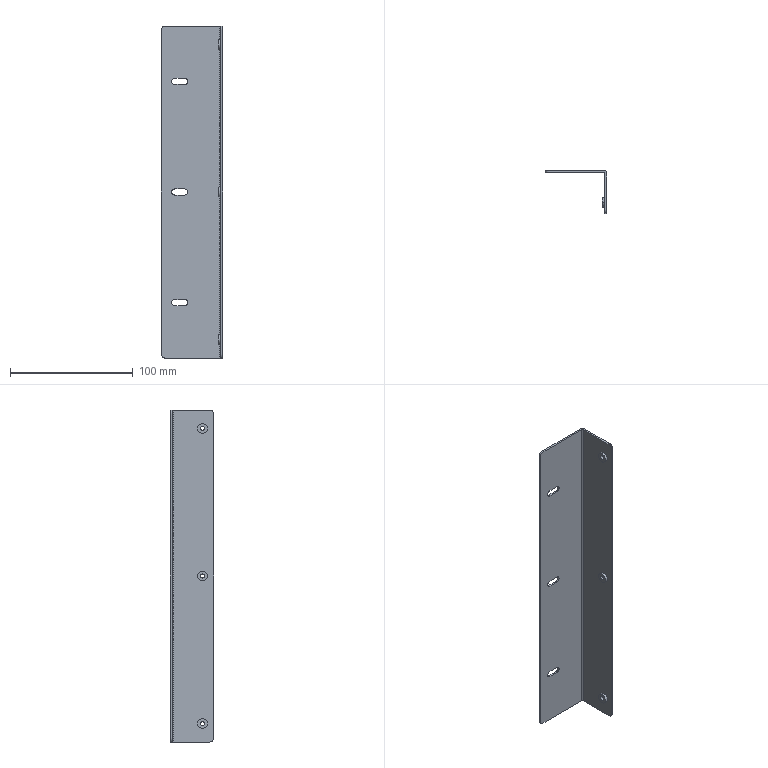Part | SolidWorks | features ICE 2, 3DProfileFeature 1, Fillet 1, FlatPattern 1, HoleWzd 1, SMBaseFlange 1, SheetMetal 1 | 1 solid | 45 faces | box 50 x 35 x 270 mm | volume 33491 mm3 | cylinder 24 | plane 21 | commonest cylinder face diameters 3.3 x6 5 x6 8 x6 6 x4 1.473 x1 4.473 x1
STEP:
#1=CARTESIAN_POINT('',(50.,-26.,-118.35));
#2=VERTEX_POINT('',#1);
#3=CARTESIAN_POINT('',(50.,-26.,-121.65));
#4=VERTEX_POINT('',#3);
#5=CARTESIAN_POINT('',(50.,-26.,-120.));
#6=DIRECTION('',(1.,0.,0.));
#7=DIRECTION('',(0.,1.,0.));
#8=AXIS2_PLACEMENT_3D('',#5,#6,#7);
#9=CIRCLE('',#8,1.65);
#10=EDGE_CURVE('',#2,#4,#9,.T.);
#11=ORIENTED_EDGE('',*,*,#10,.T.);
#12=CARTESIAN_POINT('',(46.5,-26.,-121.65));
#13=VERTEX_POINT('',#12);
#14=CARTESIAN_POINT('',(46.5,-26.,-121.65));
#15=DIRECTION('',(-1.,0.,0.));
#16=VECTOR('',#15,1000.);
#17=LINE('',#14,#16);
#18=EDGE_CURVE('',#4,#13,#17,.T.);
#19=ORIENTED_EDGE('',*,*,#18,.T.);
#20=CARTESIAN_POINT('',(46.5,-26.,-118.35));
#21=VERTEX_POINT('',#20);
#22=CARTESIAN_POINT('',(46.5,-26.,-120.));
#23=DIRECTION('',(-1.,0.,0.));
#24=DIRECTION('',(0.,0.,1.));
#25=AXIS2_PLACEMENT_3D('',#22,#23,#24);
#26=CIRCLE('',#25,1.65);
#27=EDGE_CURVE('',#13,#21,#26,.T.);
#28=ORIENTED_EDGE('',*,*,#27,.T.);
#29=CARTESIAN_POINT('',(46.5,-26.,-118.35));
#30=DIRECTION('',(-1.,0.,0.));
#31=VECTOR('',#30,1000.);
#32=LINE('',#29,#31);
#33=EDGE_CURVE('',#2,#21,#32,.T.);
#34=ORIENTED_EDGE('',*,*,#33,.F.);
#35=EDGE_LOOP('',(#11,#19,#28,#34));
#36=FACE_OUTER_BOUND('',#35,.T.);
#37=CARTESIAN_POINT('',(46.5,-26.,-120.));
#38=DIRECTION('',(-1.,0.,0.));
#39=DIRECTION('',(0.,0.,1.));
#40=AXIS2_PLACEMENT_3D('',#37,#38,#39);
#41=CYLINDRICAL_SURFACE('',#40,1.65);
#42=ADVANCED_FACE('',(#36),#41,.F.);
#43=CARTESIAN_POINT('',(50.,-26.,1.65));
#44=VERTEX_POINT('',#43);
#45=CARTESIAN_POINT('',(50.,-26.,-1.65));
#46=VERTEX_POINT('',#45);
#47=CARTESIAN_POINT('',(50.,-26.,0.));
#48=DIRECTION('',(1.,0.,0.));
#49=DIRECTION('',(0.,1.,0.));
#50=AXIS2_PLACEMENT_3D('',#47,#48,#49);
#51=CIRCLE('',#50,1.65);
#52=EDGE_CURVE('',#44,#46,#51,.T.);
#53=ORIENTED_EDGE('',*,*,#52,.T.);
#54=CARTESIAN_POINT('',(46.5,-26.,-1.65));
#55=VERTEX_POINT('',#54);
#56=CARTESIAN_POINT('',(46.5,-26.,-1.65));
#57=DIRECTION('',(-1.,0.,0.));
#58=VECTOR('',#57,1000.);
#59=LINE('',#56,#58);
#60=EDGE_CURVE('',#46,#55,#59,.T.);
#61=ORIENTED_EDGE('',*,*,#60,.T.);
#62=CARTESIAN_POINT('',(46.5,-26.,1.65));
#63=VERTEX_POINT('',#62);
#64=CARTESIAN_POINT('',(46.5,-26.,0.));
#65=DIRECTION('',(-1.,0.,0.));
#66=DIRECTION('',(0.,0.,1.));
#67=AXIS2_PLACEMENT_3D('',#64,#65,#66);
#68=CIRCLE('',#67,1.65);
#69=EDGE_CURVE('',#55,#63,#68,.T.);
#70=ORIENTED_EDGE('',*,*,#69,.T.);
#71=CARTESIAN_POINT('',(46.5,-26.,1.65));
#72=DIRECTION('',(-1.,0.,0.));
#73=VECTOR('',#72,1000.);
#74=LINE('',#71,#73);
#75=EDGE_CURVE('',#44,#63,#74,.T.);
#76=ORIENTED_EDGE('',*,*,#75,.F.);
#77=EDGE_LOOP('',(#53,#61,#70,#76));
#78=FACE_OUTER_BOUND('',#77,.T.);
#79=CARTESIAN_POINT('',(46.5,-26.,0.));
#80=DIRECTION('',(-1.,0.,0.));
#81=DIRECTION('',(0.,0.,1.));
#82=AXIS2_PLACEMENT_3D('',#79,#80,#81);
#83=CYLINDRICAL_SURFACE('',#82,1.65);
#84=ADVANCED_FACE('',(#78),#83,.F.);
#85=CARTESIAN_POINT('',(50.,-26.,121.65));
#86=VERTEX_POINT('',#85);
#87=CARTESIAN_POINT('',(50.,-26.,118.35));
#88=VERTEX_POINT('',#87);
#89=CARTESIAN_POINT('',(50.,-26.,120.));
#90=DIRECTION('',(1.,0.,0.));
#91=DIRECTION('',(0.,1.,0.));
#92=AXIS2_PLACEMENT_3D('',#89,#90,#91);
#93=CIRCLE('',#92,1.65);
#94=EDGE_CURVE('',#86,#88,#93,.T.);
#95=ORIENTED_EDGE('',*,*,#94,.T.);
#96=CARTESIAN_POINT('',(46.5,-26.,118.35));
#97=VERTEX_POINT('',#96);
#98=CARTESIAN_POINT('',(46.5,-26.,118.35));
#99=DIRECTION('',(-1.,0.,0.));
#100=VECTOR('',#99,1000.);
#101=LINE('',#98,#100);
#102=EDGE_CURVE('',#88,#97,#101,.T.);
#103=ORIENTED_EDGE('',*,*,#102,.T.);
#104=CARTESIAN_POINT('',(46.5,-26.,121.65));
#105=VERTEX_POINT('',#104);
#106=CARTESIAN_POINT('',(46.5,-26.,120.));
#107=DIRECTION('',(-1.,0.,0.));
#108=DIRECTION('',(0.,0.,1.));
#109=AXIS2_PLACEMENT_3D('',#106,#107,#108);
#110=CIRCLE('',#109,1.65);
#111=EDGE_CURVE('',#97,#105,#110,.T.);
#112=ORIENTED_EDGE('',*,*,#111,.T.);
#113=CARTESIAN_POINT('',(46.5,-26.,121.65));
#114=DIRECTION('',(-1.,0.,0.));
#115=VECTOR('',#114,1000.);
#116=LINE('',#113,#115);
#117=EDGE_CURVE('',#86,#105,#116,.T.);
#118=ORIENTED_EDGE('',*,*,#117,.F.);
#119=EDGE_LOOP('',(#95,#103,#112,#118));
#120=FACE_OUTER_BOUND('',#119,.T.);
#121=CARTESIAN_POINT('',(46.5,-26.,120.));
#122=DIRECTION('',(-1.,0.,0.));
#123=DIRECTION('',(0.,0.,1.));
#124=AXIS2_PLACEMENT_3D('',#121,#122,#123);
#125=CYLINDRICAL_SURFACE('',#124,1.65);
#126=ADVANCED_FACE('',(#120),#125,.F.);
#127=CARTESIAN_POINT('',(46.5,-26.,-124.));
#128=VERTEX_POINT('',#127);
#129=CARTESIAN_POINT('',(46.5,-26.,-116.));
#130=VERTEX_POINT('',#129);
#131=CARTESIAN_POINT('',(46.5,-26.,-120.));
#132=DIRECTION('',(1.,0.,0.));
#133=DIRECTION('',(0.,0.,1.));
#134=AXIS2_PLACEMENT_3D('',#131,#132,#133);
#135=CIRCLE('',#134,4.);
#136=EDGE_CURVE('',#128,#130,#135,.T.);
#137=ORIENTED_EDGE('',*,*,#136,.T.);
#138=CARTESIAN_POINT('',(48.5,-26.,-116.));
#139=VERTEX_POINT('',#138);
#140=CARTESIAN_POINT('',(46.5,-26.,-116.));
#141=DIRECTION('',(1.,0.,0.));
#142=VECTOR('',#141,1000.);
#143=LINE('',#140,#142);
#144=EDGE_CURVE('',#130,#139,#143,.T.);
#145=ORIENTED_EDGE('',*,*,#144,.T.);
#146=CARTESIAN_POINT('',(48.5,-26.,-124.));
#147=VERTEX_POINT('',#146);
#148=CARTESIAN_POINT('',(48.5,-26.,-120.));
#149=DIRECTION('',(1.,0.,0.));
#150=DIRECTION('',(0.,1.,0.));
#151=AXIS2_PLACEMENT_3D('',#148,#149,#150);
#152=CIRCLE('',#151,4.);
#153=EDGE_CURVE('',#147,#139,#152,.T.);
#154=ORIENTED_EDGE('',*,*,#153,.F.);
#155=CARTESIAN_POINT('',(46.5,-26.,-124.));
#156=DIRECTION('',(1.,0.,0.));
#157=VECTOR('',#156,1000.);
#158=LINE('',#155,#157);
#159=EDGE_CURVE('',#128,#147,#158,.T.);
#160=ORIENTED_EDGE('',*,*,#159,.F.);
#161=EDGE_LOOP('',(#137,#145,#154,#160));
#162=FACE_OUTER_BOUND('',#161,.T.);
#163=CARTESIAN_POINT('',(46.5,-26.,-120.));
#164=DIRECTION('',(1.,0.,0.));
#165=DIRECTION('',(0.,0.,-1.));
#166=AXIS2_PLACEMENT_3D('',#163,#164,#165);
#167=CYLINDRICAL_SURFACE('',#166,4.);
#168=ADVANCED_FACE('',(#162),#167,.T.);
#169=CARTESIAN_POINT('',(46.5,-26.,116.));
#170=VERTEX_POINT('',#169);
#171=CARTESIAN_POINT('',(46.5,-26.,124.));
#172=VERTEX_POINT('',#171);
#173=CARTESIAN_POINT('',(46.5,-26.,120.));
#174=DIRECTION('',(1.,0.,0.));
#175=DIRECTION('',(0.,0.,-1.));
#176=AXIS2_PLACEMENT_3D('',#173,#174,#175);
#177=CIRCLE('',#176,4.);
#178=EDGE_CURVE('',#170,#172,#177,.T.);
#179=ORIENTED_EDGE('',*,*,#178,.T.);
#180=CARTESIAN_POINT('',(48.5,-26.,124.));
#181=VERTEX_POINT('',#180);
#182=CARTESIAN_POINT('',(46.5,-26.,124.));
#183=DIRECTION('',(1.,0.,0.));
#184=VECTOR('',#183,1000.);
#185=LINE('',#182,#184);
#186=EDGE_CURVE('',#172,#181,#185,.T.);
#187=ORIENTED_EDGE('',*,*,#186,.T.);
#188=CARTESIAN_POINT('',(48.5,-26.,116.));
#189=VERTEX_POINT('',#188);
#190=CARTESIAN_POINT('',(48.5,-26.,120.));
#191=DIRECTION('',(1.,0.,0.));
#192=DIRECTION('',(0.,1.,0.));
#193=AXIS2_PLACEMENT_3D('',#190,#191,#192);
#194=CIRCLE('',#193,4.);
#195=EDGE_CURVE('',#189,#181,#194,.T.);
#196=ORIENTED_EDGE('',*,*,#195,.F.);
#197=CARTESIAN_POINT('',(46.5,-26.,116.));
#198=DIRECTION('',(1.,0.,0.));
#199=VECTOR('',#198,1000.);
#200=LINE('',#197,#199);
#201=EDGE_CURVE('',#170,#189,#200,.T.);
#202=ORIENTED_EDGE('',*,*,#201,.F.);
#203=EDGE_LOOP('',(#179,#187,#196,#202));
#204=FACE_OUTER_BOUND('',#203,.T.);
#205=CARTESIAN_POINT('',(46.5,-26.,120.));
#206=DIRECTION('',(1.,0.,0.));
#207=DIRECTION('',(0.,0.,-1.));
#208=AXIS2_PLACEMENT_3D('',#205,#206,#207);
#209=CYLINDRICAL_SURFACE('',#208,4.);
#210=ADVANCED_FACE('',(#204),#209,.T.);
#211=CARTESIAN_POINT('',(46.5,-26.,-4.));
#212=VERTEX_POINT('',#211);
#213=CARTESIAN_POINT('',(46.5,-26.,4.));
#214=VERTEX_POINT('',#213);
#215=CARTESIAN_POINT('',(46.5,-26.,0.));
#216=DIRECTION('',(1.,0.,0.));
#217=DIRECTION('',(0.,0.,-1.));
#218=AXIS2_PLACEMENT_3D('',#215,#216,#217);
#219=CIRCLE('',#218,4.);
#220=EDGE_CURVE('',#212,#214,#219,.T.);
#221=ORIENTED_EDGE('',*,*,#220,.T.);
#222=CARTESIAN_POINT('',(48.5,-26.,4.));
#223=VERTEX_POINT('',#222);
#224=CARTESIAN_POINT('',(46.5,-26.,4.));
#225=DIRECTION('',(1.,0.,0.));
#226=VECTOR('',#225,1000.);
#227=LINE('',#224,#226);
#228=EDGE_CURVE('',#214,#223,#227,.T.);
#229=ORIENTED_EDGE('',*,*,#228,.T.);
#230=CARTESIAN_POINT('',(48.5,-26.,-4.));
#231=VERTEX_POINT('',#230);
#232=CARTESIAN_POINT('',(48.5,-26.,0.));
#233=DIRECTION('',(1.,0.,0.));
#234=DIRECTION('',(0.,1.,0.));
#235=AXIS2_PLACEMENT_3D('',#232,#233,#234);
#236=CIRCLE('',#235,4.);
#237=EDGE_CURVE('',#231,#223,#236,.T.);
#238=ORIENTED_EDGE('',*,*,#237,.F.);
#239=CARTESIAN_POINT('',(46.5,-26.,-4.));
#240=DIRECTION('',(1.,0.,0.));
#241=VECTOR('',#240,1000.);
#242=LINE('',#239,#241);
#243=EDGE_CURVE('',#212,#231,#242,.T.);
#244=ORIENTED_EDGE('',*,*,#243,.F.);
#245=EDGE_LOOP('',(#221,#229,#238,#244));
#246=FACE_OUTER_BOUND('',#245,.T.);
#247=CARTESIAN_POINT('',(46.5,-26.,0.));
#248=DIRECTION('',(1.,0.,0.));
#249=DIRECTION('',(0.,0.,-1.));
#250=AXIS2_PLACEMENT_3D('',#247,#248,#249);
#251=CYLINDRICAL_SURFACE('',#250,4.);
#252=ADVANCED_FACE('',(#246),#251,.T.);
#253=ORIENTED_EDGE('',*,*,#178,.F.);
#254=CARTESIAN_POINT('',(46.5,-26.,120.));
#255=DIRECTION('',(1.,0.,0.));
#256=DIRECTION('',(0.,0.,-1.));
#257=AXIS2_PLACEMENT_3D('',#254,#255,#256);
#258=CIRCLE('',#257,4.);
#259=EDGE_CURVE('',#172,#170,#258,.T.);
#260=ORIENTED_EDGE('',*,*,#259,.F.);
#261=EDGE_LOOP('',(#253,#260));
#262=FACE_OUTER_BOUND('',#261,.T.);
#263=CARTESIAN_POINT('',(46.5,-26.,120.));
#264=DIRECTION('',(-1.,0.,0.));
#265=DIRECTION('',(0.,0.,1.));
#266=AXIS2_PLACEMENT_3D('',#263,#264,#265);
#267=CIRCLE('',#266,1.65);
#268=EDGE_CURVE('',#105,#97,#267,.T.);
#269=ORIENTED_EDGE('',*,*,#268,.F.);
#270=ORIENTED_EDGE('',*,*,#111,.F.);
#271=EDGE_LOOP('',(#269,#270));
#272=FACE_BOUND('',#271,.T.);
#273=CARTESIAN_POINT('',(46.5,-26.,120.));
#274=DIRECTION('',(1.,0.,0.));
#275=DIRECTION('',(0.,0.,-1.));
#276=AXIS2_PLACEMENT_3D('',#273,#274,#275);
#277=PLANE('',#276);
#278=ADVANCED_FACE('',(#262,#272),#277,.F.);
#279=CARTESIAN_POINT('',(0.,0.,132.));
#280=VERTEX_POINT('',#279);
#281=CARTESIAN_POINT('',(0.,0.,-132.));
#282=VERTEX_POINT('',#281);
#283=CARTESIAN_POINT('',(0.,0.,135.));
#284=DIRECTION('',(0.,0.,-1.));
#285=VECTOR('',#284,1000.);
#286=LINE('',#283,#285);
#287=EDGE_CURVE('',#280,#282,#286,.T.);
#288=ORIENTED_EDGE('',*,*,#287,.F.);
#289=CARTESIAN_POINT('',(3.,0.,135.));
#290=VERTEX_POINT('',#289);
#291=CARTESIAN_POINT('',(3.,0.,132.));
#292=DIRECTION('',(0.,1.,0.));
#293=DIRECTION('',(0.,0.,1.));
#294=AXIS2_PLACEMENT_3D('',#291,#292,#293);
#295=CIRCLE('',#294,3.);
#296=EDGE_CURVE('',#280,#290,#295,.T.);
#297=ORIENTED_EDGE('',*,*,#296,.T.);
#298=CARTESIAN_POINT('',(47.763,0.,135.));
#299=VERTEX_POINT('',#298);
#300=CARTESIAN_POINT('',(0.,0.,135.));
#301=DIRECTION('',(1.,0.,0.));
#302=VECTOR('',#301,1000.);
#303=LINE('',#300,#302);
#304=EDGE_CURVE('',#290,#299,#303,.T.);
#305=ORIENTED_EDGE('',*,*,#304,.T.);
#306=CARTESIAN_POINT('',(47.763,0.,-135.));
#307=VERTEX_POINT('',#306);
#308=CARTESIAN_POINT('',(47.763,0.,135.));
#309=DIRECTION('',(0.,0.,-1.));
#310=VECTOR('',#309,1000.);
#311=LINE('',#308,#310);
#312=EDGE_CURVE('',#299,#307,#311,.T.);
#313=ORIENTED_EDGE('',*,*,#312,.T.);
#314=CARTESIAN_POINT('',(3.,0.,-135.));
#315=VERTEX_POINT('',#314);
#316=CARTESIAN_POINT('',(0.,0.,-135.));
#317=DIRECTION('',(1.,0.,0.));
#318=VECTOR('',#317,1000.);
#319=LINE('',#316,#318);
#320=EDGE_CURVE('',#315,#307,#319,.T.);
#321=ORIENTED_EDGE('',*,*,#320,.F.);
#322=CARTESIAN_POINT('',(3.,0.,-132.));
#323=DIRECTION('',(0.,1.,0.));
#324=DIRECTION('',(0.,0.,1.));
#325=AXIS2_PLACEMENT_3D('',#322,#323,#324);
#326=CIRCLE('',#325,3.);
#327=EDGE_CURVE('',#315,#282,#326,.T.);
#328=ORIENTED_EDGE('',*,*,#327,.T.);
#329=EDGE_LOOP('',(#288,#297,#305,#313,#321,#328));
#330=FACE_OUTER_BOUND('',#329,.T.);
#331=CARTESIAN_POINT('',(11.,0.,87.5));
#332=VERTEX_POINT('',#331);
#333=CARTESIAN_POINT('',(19.,0.,87.5));
#334=VERTEX_POINT('',#333);
#335=CARTESIAN_POINT('',(19.,0.,87.5));
#336=DIRECTION('',(1.,0.,0.));
#337=VECTOR('',#336,1000.);
#338=LINE('',#335,#337);
#339=EDGE_CURVE('',#332,#334,#338,.T.);
#340=ORIENTED_EDGE('',*,*,#339,.T.);
#341=CARTESIAN_POINT('',(19.,0.,92.5));
#342=VERTEX_POINT('',#341);
#343=CARTESIAN_POINT('',(19.,0.,90.));
#344=DIRECTION('',(0.,-1.,0.));
#345=DIRECTION('',(0.,0.,1.));
#346=AXIS2_PLACEMENT_3D('',#343,#344,#345);
#347=CIRCLE('',#346,2.5);
#348=EDGE_CURVE('',#334,#342,#347,.T.);
#349=ORIENTED_EDGE('',*,*,#348,.T.);
#350=CARTESIAN_POINT('',(11.,0.,92.5));
#351=VERTEX_POINT('',#350);
#352=CARTESIAN_POINT('',(19.,0.,92.5));
#353=DIRECTION('',(-1.,0.,0.));
#354=VECTOR('',#353,1000.);
#355=LINE('',#352,#354);
#356=EDGE_CURVE('',#342,#351,#355,.T.);
#357=ORIENTED_EDGE('',*,*,#356,.T.);
#358=CARTESIAN_POINT('',(11.,0.,90.));
#359=DIRECTION('',(0.,-1.,0.));
#360=DIRECTION('',(0.,0.,1.));
#361=AXIS2_PLACEMENT_3D('',#358,#359,#360);
#362=CIRCLE('',#361,2.5);
#363=EDGE_CURVE('',#351,#332,#362,.T.);
#364=ORIENTED_EDGE('',*,*,#363,.T.);
#365=EDGE_LOOP('',(#340,#349,#357,#364));
#366=FACE_BOUND('',#365,.T.);
#367=CARTESIAN_POINT('',(11.,0.,-2.5));
#368=VERTEX_POINT('',#367);
#369=CARTESIAN_POINT('',(19.,0.,-2.5));
#370=VERTEX_POINT('',#369);
#371=CARTESIAN_POINT('',(19.,0.,-2.5));
#372=DIRECTION('',(1.,0.,0.));
#373=VECTOR('',#372,1000.);
#374=LINE('',#371,#373);
#375=EDGE_CURVE('',#368,#370,#374,.T.);
#376=ORIENTED_EDGE('',*,*,#375,.T.);
#377=CARTESIAN_POINT('',(19.,0.,2.5));
#378=VERTEX_POINT('',#377);
#379=CARTESIAN_POINT('',(19.,0.,0.));
#380=DIRECTION('',(0.,-1.,0.));
#381=DIRECTION('',(0.,0.,-1.));
#382=AXIS2_PLACEMENT_3D('',#379,#380,#381);
#383=CIRCLE('',#382,2.5);
#384=EDGE_CURVE('',#370,#378,#383,.T.);
#385=ORIENTED_EDGE('',*,*,#384,.T.);
#386=CARTESIAN_POINT('',(11.,0.,2.5));
#387=VERTEX_POINT('',#386);
#388=CARTESIAN_POINT('',(19.,0.,2.5));
#389=DIRECTION('',(-1.,0.,0.));
#390=VECTOR('',#389,1000.);
#391=LINE('',#388,#390);
#392=EDGE_CURVE('',#378,#387,#391,.T.);
#393=ORIENTED_EDGE('',*,*,#392,.T.);
#394=CARTESIAN_POINT('',(11.,0.,0.));
#395=DIRECTION('',(0.,-1.,0.));
#396=DIRECTION('',(0.,0.,-1.));
#397=AXIS2_PLACEMENT_3D('',#394,#395,#396);
#398=CIRCLE('',#397,2.5);
#399=EDGE_CURVE('',#387,#368,#398,.T.);
#400=ORIENTED_EDGE('',*,*,#399,.T.);
#401=EDGE_LOOP('',(#376,#385,#393,#400));
#402=FACE_BOUND('',#401,.T.);
#403=CARTESIAN_POINT('',(11.,0.,-92.5));
#404=VERTEX_POINT('',#403);
#405=CARTESIAN_POINT('',(19.,0.,-92.5));
#406=VERTEX_POINT('',#405);
#407=CARTESIAN_POINT('',(19.,0.,-92.5));
#408=DIRECTION('',(1.,0.,0.));
#409=VECTOR('',#408,1000.);
#410=LINE('',#407,#409);
#411=EDGE_CURVE('',#404,#406,#410,.T.);
#412=ORIENTED_EDGE('',*,*,#411,.T.);
#413=CARTESIAN_POINT('',(19.,0.,-87.5));
#414=VERTEX_POINT('',#413);
#415=CARTESIAN_POINT('',(19.,0.,-90.));
#416=DIRECTION('',(0.,-1.,0.));
#417=DIRECTION('',(0.,0.,-1.));
#418=AXIS2_PLACEMENT_3D('',#415,#416,#417);
#419=CIRCLE('',#418,2.5);
#420=EDGE_CURVE('',#406,#414,#419,.T.);
#421=ORIENTED_EDGE('',*,*,#420,.T.);
#422=CARTESIAN_POINT('',(11.,0.,-87.5));
#423=VERTEX_POINT('',#422);
#424=CARTESIAN_POINT('',(19.,0.,-87.5));
#425=DIRECTION('',(-1.,0.,0.));
#426=VECTOR('',#425,1000.);
#427=LINE('',#424,#426);
#428=EDGE_CURVE('',#414,#423,#427,.T.);
#429=ORIENTED_EDGE('',*,*,#428,.T.);
#430=CARTESIAN_POINT('',(11.,0.,-90.));
#431=DIRECTION('',(0.,-1.,0.));
#432=DIRECTION('',(0.,0.,-1.));
#433=AXIS2_PLACEMENT_3D('',#430,#431,#432);
#434=CIRCLE('',#433,2.5);
#435=EDGE_CURVE('',#423,#404,#434,.T.);
#436=ORIENTED_EDGE('',*,*,#435,.T.);
#437=EDGE_LOOP('',(#412,#421,#429,#436));
#438=FACE_BOUND('',#437,.T.);
#439=CARTESIAN_POINT('',(0.,0.,135.));
#440=DIRECTION('',(0.,1.,0.));
#441=DIRECTION('',(0.,0.,1.));
#442=AXIS2_PLACEMENT_3D('',#439,#440,#441);
#443=PLANE('',#442);
#444=ADVANCED_FACE('',(#330,#366,#402,#438),#443,.T.);
#445=CARTESIAN_POINT('',(19.,-1.5,-2.5));
#446=VERTEX_POINT('',#445);
#447=CARTESIAN_POINT('',(19.,-1.5,2.5));
#448=VERTEX_POINT('',#447);
#449=CARTESIAN_POINT('',(19.,-1.5,0.));
#450=DIRECTION('',(0.,-1.,0.));
#451=DIRECTION('',(0.,0.,1.));
#452=AXIS2_PLACEMENT_3D('',#449,#450,#451);
#453=CIRCLE('',#452,2.5);
#454=EDGE_CURVE('',#446,#448,#453,.T.);
#455=ORIENTED_EDGE('',*,*,#454,.F.);
#456=CARTESIAN_POINT('',(11.,-1.5,-2.5));
#457=VERTEX_POINT('',#456);
#458=CARTESIAN_POINT('',(0.,-1.5,-2.5));
#459=DIRECTION('',(1.,0.,0.));
#460=VECTOR('',#459,1000.);
#461=LINE('',#458,#460);
#462=EDGE_CURVE('',#457,#446,#461,.T.);
#463=ORIENTED_EDGE('',*,*,#462,.F.);
#464=CARTESIAN_POINT('',(11.,-1.5,2.5));
#465=VERTEX_POINT('',#464);
#466=CARTESIAN_POINT('',(11.,-1.5,0.));
#467=DIRECTION('',(0.,-1.,0.));
#468=DIRECTION('',(0.,0.,1.));
#469=AXIS2_PLACEMENT_3D('',#466,#467,#468);
#470=CIRCLE('',#469,2.5);
#471=EDGE_CURVE('',#465,#457,#470,.T.);
#472=ORIENTED_EDGE('',*,*,#471,.F.);
#473=CARTESIAN_POINT('',(0.,-1.5,2.5));
#474=DIRECTION('',(-1.,0.,0.));
#475=VECTOR('',#474,1000.);
#476=LINE('',#473,#475);
#477=EDGE_CURVE('',#448,#465,#476,.T.);
#478=ORIENTED_EDGE('',*,*,#477,.F.);
#479=EDGE_LOOP('',(#455,#463,#472,#478));
#480=FACE_BOUND('',#479,.T.);
#481=CARTESIAN_POINT('',(3.,-1.5,135.));
#482=VERTEX_POINT('',#481);
#483=CARTESIAN_POINT('',(47.763,-1.5,135.));
#484=VERTEX_POINT('',#483);
#485=CARTESIAN_POINT('',(0.,-1.5,135.));
#486=DIRECTION('',(1.,0.,0.));
#487=VECTOR('',#486,1000.);
#488=LINE('',#485,#487);
#489=EDGE_CURVE('',#482,#484,#488,.T.);
#490=ORIENTED_EDGE('',*,*,#489,.F.);
#491=CARTESIAN_POINT('',(0.,-1.5,132.));
#492=VERTEX_POINT('',#491);
#493=CARTESIAN_POINT('',(3.,-1.5,132.));
#494=DIRECTION('',(0.,-1.,0.));
#495=DIRECTION('',(0.,0.,1.));
#496=AXIS2_PLACEMENT_3D('',#493,#494,#495);
#497=CIRCLE('',#496,3.);
#498=EDGE_CURVE('',#482,#492,#497,.T.);
#499=ORIENTED_EDGE('',*,*,#498,.T.);
#500=CARTESIAN_POINT('',(0.,-1.5,-132.));
#501=VERTEX_POINT('',#500);
#502=CARTESIAN_POINT('',(0.,-1.5,135.));
#503=DIRECTION('',(0.,0.,-1.));
#504=VECTOR('',#503,1000.);
#505=LINE('',#502,#504);
#506=EDGE_CURVE('',#492,#501,#505,.T.);
#507=ORIENTED_EDGE('',*,*,#506,.T.);
#508=CARTESIAN_POINT('',(3.,-1.5,-135.));
#509=VERTEX_POINT('',#508);
#510=CARTESIAN_POINT('',(3.,-1.5,-132.));
#511=DIRECTION('',(0.,-1.,0.));
#512=DIRECTION('',(0.,0.,1.));
#513=AXIS2_PLACEMENT_3D('',#510,#511,#512);
#514=CIRCLE('',#513,3.);
#515=EDGE_CURVE('',#501,#509,#514,.T.);
#516=ORIENTED_EDGE('',*,*,#515,.T.);
#517=CARTESIAN_POINT('',(47.763,-1.5,-135.));
#518=VERTEX_POINT('',#517);
#519=CARTESIAN_POINT('',(0.,-1.5,-135.));
#520=DIRECTION('',(1.,0.,0.));
#521=VECTOR('',#520,1000.);
#522=LINE('',#519,#521);
#523=EDGE_CURVE('',#509,#518,#522,.T.);
#524=ORIENTED_EDGE('',*,*,#523,.T.);
#525=CARTESIAN_POINT('',(47.763,-1.5,135.));
#526=DIRECTION('',(0.,0.,-1.));
#527=VECTOR('',#526,1000.);
#528=LINE('',#525,#527);
#529=EDGE_CURVE('',#484,#518,#528,.T.);
#530=ORIENTED_EDGE('',*,*,#529,.F.);
#531=EDGE_LOOP('',(#490,#499,#507,#516,#524,#530));
#532=FACE_OUTER_BOUND('',#531,.T.);
#533=CARTESIAN_POINT('',(19.,-1.5,87.5));
#534=VERTEX_POINT('',#533);
#535=CARTESIAN_POINT('',(19.,-1.5,92.5));
#536=VERTEX_POINT('',#535);
#537=CARTESIAN_POINT('',(19.,-1.5,90.));
#538=DIRECTION('',(0.,-1.,0.));
#539=DIRECTION('',(0.,0.,1.));
#540=AXIS2_PLACEMENT_3D('',#537,#538,#539);
#541=CIRCLE('',#540,2.5);
#542=EDGE_CURVE('',#534,#536,#541,.T.);
#543=ORIENTED_EDGE('',*,*,#542,.F.);
#544=CARTESIAN_POINT('',(11.,-1.5,87.5));
#545=VERTEX_POINT('',#544);
#546=CARTESIAN_POINT('',(0.,-1.5,87.5));
#547=DIRECTION('',(1.,0.,0.));
#548=VECTOR('',#547,1000.);
#549=LINE('',#546,#548);
#550=EDGE_CURVE('',#545,#534,#549,.T.);
#551=ORIENTED_EDGE('',*,*,#550,.F.);
#552=CARTESIAN_POINT('',(11.,-1.5,92.5));
#553=VERTEX_POINT('',#552);
#554=CARTESIAN_POINT('',(11.,-1.5,90.));
#555=DIRECTION('',(0.,-1.,0.));
#556=DIRECTION('',(0.,0.,1.));
#557=AXIS2_PLACEMENT_3D('',#554,#555,#556);
#558=CIRCLE('',#557,2.5);
#559=EDGE_CURVE('',#553,#545,#558,.T.);
#560=ORIENTED_EDGE('',*,*,#559,.F.);
#561=CARTESIAN_POINT('',(0.,-1.5,92.5));
#562=DIRECTION('',(-1.,0.,0.));
#563=VECTOR('',#562,1000.);
#564=LINE('',#561,#563);
#565=EDGE_CURVE('',#536,#553,#564,.T.);
#566=ORIENTED_EDGE('',*,*,#565,.F.);
#567=EDGE_LOOP('',(#543,#551,#560,#566));
#568=FACE_BOUND('',#567,.T.);
#569=CARTESIAN_POINT('',(19.,-1.5,-92.5));
#570=VERTEX_POINT('',#569);
#571=CARTESIAN_POINT('',(19.,-1.5,-87.5));
#572=VERTEX_POINT('',#571);
#573=CARTESIAN_POINT('',(19.,-1.5,-90.));
#574=DIRECTION('',(0.,-1.,0.));
#575=DIRECTION('',(0.,0.,1.));
#576=AXIS2_PLACEMENT_3D('',#573,#574,#575);
#577=CIRCLE('',#576,2.5);
#578=EDGE_CURVE('',#570,#572,#577,.T.);
#579=ORIENTED_EDGE('',*,*,#578,.F.);
#580=CARTESIAN_POINT('',(11.,-1.5,-92.5));
#581=VERTEX_POINT('',#580);
#582=CARTESIAN_POINT('',(0.,-1.5,-92.5));
#583=DIRECTION('',(1.,0.,0.));
#584=VECTOR('',#583,1000.);
#585=LINE('',#582,#584);
#586=EDGE_CURVE('',#581,#570,#585,.T.);
#587=ORIENTED_EDGE('',*,*,#586,.F.);
#588=CARTESIAN_POINT('',(11.,-1.5,-87.5));
#589=VERTEX_POINT('',#588);
#590=CARTESIAN_POINT('',(11.,-1.5,-90.));
#591=DIRECTION('',(0.,-1.,0.));
#592=DIRECTION('',(0.,0.,1.));
#593=AXIS2_PLACEMENT_3D('',#590,#591,#592);
#594=CIRCLE('',#593,2.5);
#595=EDGE_CURVE('',#589,#581,#594,.T.);
#596=ORIENTED_EDGE('',*,*,#595,.F.);
#597=CARTESIAN_POINT('',(0.,-1.5,-87.5));
#598=DIRECTION('',(-1.,0.,0.));
#599=VECTOR('',#598,1000.);
#600=LINE('',#597,#599);
#601=EDGE_CURVE('',#572,#589,#600,.T.);
#602=ORIENTED_EDGE('',*,*,#601,.F.);
#603=EDGE_LOOP('',(#579,#587,#596,#602));
#604=FACE_BOUND('',#603,.T.);
#605=CARTESIAN_POINT('',(0.,-1.5,135.));
#606=DIRECTION('',(0.,1.,0.));
#607=DIRECTION('',(0.,0.,1.));
#608=AXIS2_PLACEMENT_3D('',#605,#606,#607);
#609=PLANE('',#608);
#610=ADVANCED_FACE('',(#480,#532,#568,#604),#609,.F.);
#611=CARTESIAN_POINT('',(50.,-2.237,135.));
#612=VERTEX_POINT('',#611);
#613=CARTESIAN_POINT('',(48.5,-2.237,135.));
#614=VERTEX_POINT('',#613);
#615=CARTESIAN_POINT('',(50.,-2.237,135.));
#616=DIRECTION('',(-1.,0.,0.));
#617=VECTOR('',#616,1000.);
#618=LINE('',#615,#617);
#619=EDGE_CURVE('',#612,#614,#618,.T.);
#620=ORIENTED_EDGE('',*,*,#619,.F.);
#621=CARTESIAN_POINT('',(47.763,-2.237,135.));
#622=DIRECTION('',(0.,0.,-1.));
#623=DIRECTION('',(1.,0.,0.));
#624=AXIS2_PLACEMENT_3D('',#621,#622,#623);
#625=CIRCLE('',#624,2.237);
#626=EDGE_CURVE('',#299,#612,#625,.T.);
#627=ORIENTED_EDGE('',*,*,#626,.F.);
#628=CARTESIAN_POINT('',(47.763,-1.5,135.));
#629=DIRECTION('',(0.,1.,0.));
#630=VECTOR('',#629,1000.);
#631=LINE('',#628,#630);
#632=EDGE_CURVE('',#484,#299,#631,.T.);
#633=ORIENTED_EDGE('',*,*,#632,.F.);
#634=CARTESIAN_POINT('',(47.763,-2.237,135.));
#635=DIRECTION('',(0.,0.,-1.));
#636=DIRECTION('',(1.,0.,0.));
#637=AXIS2_PLACEMENT_3D('',#634,#635,#636);
#638=CIRCLE('',#637,0.7366);
#639=EDGE_CURVE('',#484,#614,#638,.T.);
#640=ORIENTED_EDGE('',*,*,#639,.T.);
#641=EDGE_LOOP('',(#620,#627,#633,#640));
#642=FACE_OUTER_BOUND('',#641,.T.);
#643=CARTESIAN_POINT('',(50.,-2.237,135.));
#644=DIRECTION('',(0.,0.,1.));
#645=DIRECTION('',(1.,0.,0.));
#646=AXIS2_PLACEMENT_3D('',#643,#644,#645);
#647=PLANE('',#646);
#648=ADVANCED_FACE('',(#642),#647,.T.);
#649=CARTESIAN_POINT('',(48.5,-32.,135.));
#650=VERTEX_POINT('',#649);
#651=CARTESIAN_POINT('',(48.5,0.,135.));
#652=DIRECTION('',(0.,-1.,0.));
#653=VECTOR('',#652,1000.);
#654=LINE('',#651,#653);
#655=EDGE_CURVE('',#614,#650,#654,.T.);
#656=ORIENTED_EDGE('',*,*,#655,.T.);
#657=CARTESIAN_POINT('',(50.,-32.,135.));
#658=VERTEX_POINT('',#657);
#659=CARTESIAN_POINT('',(47.763,-32.,135.));
#660=DIRECTION('',(1.,0.,0.));
#661=VECTOR('',#660,1000.);
#662=LINE('',#659,#661);
#663=EDGE_CURVE('',#650,#658,#662,.T.);
#664=ORIENTED_EDGE('',*,*,#663,.T.);
#665=CARTESIAN_POINT('',(50.,0.,135.));
#666=DIRECTION('',(0.,-1.,0.));
#667=VECTOR('',#666,1000.);
#668=LINE('',#665,#667);
#669=EDGE_CURVE('',#612,#658,#668,.T.);
#670=ORIENTED_EDGE('',*,*,#669,.F.);
#671=ORIENTED_EDGE('',*,*,#619,.T.);
#672=EDGE_LOOP('',(#656,#664,#670,#671));
#673=FACE_OUTER_BOUND('',#672,.T.);
#674=CARTESIAN_POINT('',(47.763,-1.5,135.));
#675=DIRECTION('',(0.,0.,1.));
#676=DIRECTION('',(1.,0.,0.));
#677=AXIS2_PLACEMENT_3D('',#674,#675,#676);
#678=PLANE('',#677);
#679=ADVANCED_FACE('',(#673),#678,.T.);
#680=CARTESIAN_POINT('',(47.763,0.,-135.));
#681=DIRECTION('',(0.,-1.,0.));
#682=VECTOR('',#681,1000.);
#683=LINE('',#680,#682);
#684=EDGE_CURVE('',#307,#518,#683,.T.);
#685=ORIENTED_EDGE('',*,*,#684,.F.);
#686=CARTESIAN_POINT('',(50.,-2.237,-135.));
#687=VERTEX_POINT('',#686);
#688=CARTESIAN_POINT('',(47.763,-2.237,-135.));
#689=DIRECTION('',(0.,0.,-1.));
#690=DIRECTION('',(1.,0.,0.));
#691=AXIS2_PLACEMENT_3D('',#688,#689,#690);
#692=CIRCLE('',#691,2.237);
#693=EDGE_CURVE('',#307,#687,#692,.T.);
#694=ORIENTED_EDGE('',*,*,#693,.T.);
#695=CARTESIAN_POINT('',(48.5,-2.237,-135.));
#696=VERTEX_POINT('',#695);
#697=CARTESIAN_POINT('',(48.5,-2.237,-135.));
#698=DIRECTION('',(1.,0.,0.));
#699=VECTOR('',#698,1000.);
#700=LINE('',#697,#699);
#701=EDGE_CURVE('',#696,#687,#700,.T.);
#702=ORIENTED_EDGE('',*,*,#701,.F.);
#703=CARTESIAN_POINT('',(47.763,-2.237,-135.));
#704=DIRECTION('',(0.,0.,-1.));
#705=DIRECTION('',(1.,0.,0.));
#706=AXIS2_PLACEMENT_3D('',#703,#704,#705);
#707=CIRCLE('',#706,0.7366);
#708=EDGE_CURVE('',#518,#696,#707,.T.);
#709=ORIENTED_EDGE('',*,*,#708,.F.);
#710=EDGE_LOOP('',(#685,#694,#702,#709));
#711=FACE_OUTER_BOUND('',#710,.T.);
#712=CARTESIAN_POINT('',(47.763,0.,-135.));
#713=DIRECTION('',(0.,0.,-1.));
#714=DIRECTION('',(-1.,0.,0.));
#715=AXIS2_PLACEMENT_3D('',#712,#713,#714);
#716=PLANE('',#715);
#717=ADVANCED_FACE('',(#711),#716,.T.);
#718=ORIENTED_EDGE('',*,*,#523,.F.);
#719=CARTESIAN_POINT('',(3.,-2.237,-135.));
#720=DIRECTION('',(0.,1.,0.));
#721=VECTOR('',#720,1000.);
#722=LINE('',#719,#721);
#723=EDGE_CURVE('',#509,#315,#722,.T.);
#724=ORIENTED_EDGE('',*,*,#723,.T.);
#725=ORIENTED_EDGE('',*,*,#320,.T.);
#726=ORIENTED_EDGE('',*,*,#684,.T.);
#727=EDGE_LOOP('',(#718,#724,#725,#726));
#728=FACE_OUTER_BOUND('',#727,.T.);
#729=CARTESIAN_POINT('',(48.5,-2.237,-135.));
#730=DIRECTION('',(0.,0.,-1.));
#731=DIRECTION('',(-1.,0.,0.));
#732=AXIS2_PLACEMENT_3D('',#729,#730,#731);
#733=PLANE('',#732);
#734=ADVANCED_FACE('',(#728),#733,.T.);
#735=ORIENTED_EDGE('',*,*,#153,.T.);
#736=CARTESIAN_POINT('',(48.5,-26.,-120.));
#737=DIRECTION('',(1.,0.,0.));
#738=DIRECTION('',(0.,1.,0.));
#739=AXIS2_PLACEMENT_3D('',#736,#737,#738);
#740=CIRCLE('',#739,4.);
#741=EDGE_CURVE('',#139,#147,#740,.T.);
#742=ORIENTED_EDGE('',*,*,#741,.T.);
#743=EDGE_LOOP('',(#735,#742));
#744=FACE_BOUND('',#743,.T.);
#745=ORIENTED_EDGE('',*,*,#195,.T.);
#746=CARTESIAN_POINT('',(48.5,-26.,120.));
#747=DIRECTION('',(1.,0.,0.));
#748=DIRECTION('',(0.,1.,0.));
#749=AXIS2_PLACEMENT_3D('',#746,#747,#748);
#750=CIRCLE('',#749,4.);
#751=EDGE_CURVE('',#181,#189,#750,.T.);
#752=ORIENTED_EDGE('',*,*,#751,.T.);
#753=EDGE_LOOP('',(#745,#752));
#754=FACE_BOUND('',#753,.T.);
#755=ORIENTED_EDGE('',*,*,#237,.T.);
#756=CARTESIAN_POINT('',(48.5,-26.,0.));
#757=DIRECTION('',(1.,0.,0.));
#758=DIRECTION('',(0.,1.,0.));
#759=AXIS2_PLACEMENT_3D('',#756,#757,#758);
#760=CIRCLE('',#759,4.);
#761=EDGE_CURVE('',#223,#231,#760,.T.);
#762=ORIENTED_EDGE('',*,*,#761,.T.);
#763=EDGE_LOOP('',(#755,#762));
#764=FACE_BOUND('',#763,.T.);
#765=CARTESIAN_POINT('',(48.5,-32.,-135.));
#766=VERTEX_POINT('',#765);
#767=CARTESIAN_POINT('',(48.5,0.,-135.));
#768=DIRECTION('',(0.,-1.,0.));
#769=VECTOR('',#768,1000.);
#770=LINE('',#767,#769);
#771=EDGE_CURVE('',#696,#766,#770,.T.);
#772=ORIENTED_EDGE('',*,*,#771,.T.);
#773=CARTESIAN_POINT('',(48.5,-35.,-132.));
#774=VERTEX_POINT('',#773);
#775=CARTESIAN_POINT('',(48.5,-32.,-132.));
#776=DIRECTION('',(-1.,0.,0.));
#777=DIRECTION('',(0.,1.,0.));
#778=AXIS2_PLACEMENT_3D('',#775,#776,#777);
#779=CIRCLE('',#778,3.);
#780=EDGE_CURVE('',#766,#774,#779,.T.);
#781=ORIENTED_EDGE('',*,*,#780,.T.);
#782=CARTESIAN_POINT('',(48.5,-35.,132.));
#783=VERTEX_POINT('',#782);
#784=CARTESIAN_POINT('',(48.5,-35.,135.));
#785=DIRECTION('',(0.,0.,-1.));
#786=VECTOR('',#785,1000.);
#787=LINE('',#784,#786);
#788=EDGE_CURVE('',#783,#774,#787,.T.);
#789=ORIENTED_EDGE('',*,*,#788,.F.);
#790=CARTESIAN_POINT('',(48.5,-32.,132.));
#791=DIRECTION('',(-1.,0.,0.));
#792=DIRECTION('',(0.,1.,0.));
#793=AXIS2_PLACEMENT_3D('',#790,#791,#792);
#794=CIRCLE('',#793,3.);
#795=EDGE_CURVE('',#783,#650,#794,.T.);
#796=ORIENTED_EDGE('',*,*,#795,.T.);
#797=ORIENTED_EDGE('',*,*,#655,.F.);
#798=CARTESIAN_POINT('',(48.5,-2.237,135.));
#799=DIRECTION('',(0.,0.,-1.));
#800=VECTOR('',#799,1000.);
#801=LINE('',#798,#800);
#802=EDGE_CURVE('',#614,#696,#801,.T.);
#803=ORIENTED_EDGE('',*,*,#802,.T.);
#804=EDGE_LOOP('',(#772,#781,#789,#796,#797,#803));
#805=FACE_OUTER_BOUND('',#804,.T.);
#806=CARTESIAN_POINT('',(48.5,0.,135.));
#807=DIRECTION('',(1.,0.,0.));
#808=DIRECTION('',(0.,1.,0.));
#809=AXIS2_PLACEMENT_3D('',#806,#807,#808);
#810=PLANE('',#809);
#811=ADVANCED_FACE('',(#744,#754,#764,#805),#810,.F.);
#812=ORIENTED_EDGE('',*,*,#788,.T.);
#813=CARTESIAN_POINT('',(50.,-35.,-132.));
#814=VERTEX_POINT('',#813);
#815=CARTESIAN_POINT('',(50.,-35.,-132.));
#816=DIRECTION('',(1.,0.,0.));
#817=VECTOR('',#816,1000.);
#818=LINE('',#815,#817);
#819=EDGE_CURVE('',#774,#814,#818,.T.);
#820=ORIENTED_EDGE('',*,*,#819,.T.);
#821=CARTESIAN_POINT('',(50.,-35.,132.));
#822=VERTEX_POINT('',#821);
#823=CARTESIAN_POINT('',(50.,-35.,135.));
#824=DIRECTION('',(0.,0.,-1.));
#825=VECTOR('',#824,1000.);
#826=LINE('',#823,#825);
#827=EDGE_CURVE('',#822,#814,#826,.T.);
#828=ORIENTED_EDGE('',*,*,#827,.F.);
#829=CARTESIAN_POINT('',(50.,-35.,132.));
#830=DIRECTION('',(-1.,0.,0.));
#831=VECTOR('',#830,1000.);
#832=LINE('',#829,#831);
#833=EDGE_CURVE('',#822,#783,#832,.T.);
#834=ORIENTED_EDGE('',*,*,#833,.T.);
#835=EDGE_LOOP('',(#812,#820,#828,#834));
#836=FACE_OUTER_BOUND('',#835,.T.);
#837=CARTESIAN_POINT('',(50.,-35.,135.));
#838=DIRECTION('',(0.,-1.,0.));
#839=DIRECTION('',(0.,0.,-1.));
#840=AXIS2_PLACEMENT_3D('',#837,#838,#839);
#841=PLANE('',#840);
#842=ADVANCED_FACE('',(#836),#841,.T.);
#843=ORIENTED_EDGE('',*,*,#10,.F.);
#844=CARTESIAN_POINT('',(50.,-26.,-120.));
#845=DIRECTION('',(1.,0.,0.));
#846=DIRECTION('',(0.,1.,0.));
#847=AXIS2_PLACEMENT_3D('',#844,#845,#846);
#848=CIRCLE('',#847,1.65);
#849=EDGE_CURVE('',#4,#2,#848,.T.);
#850=ORIENTED_EDGE('',*,*,#849,.F.);
#851=EDGE_LOOP('',(#843,#850));
#852=FACE_BOUND('',#851,.T.);
#853=ORIENTED_EDGE('',*,*,#52,.F.);
#854=CARTESIAN_POINT('',(50.,-26.,0.));
#855=DIRECTION('',(1.,0.,0.));
#856=DIRECTION('',(0.,1.,0.));
#857=AXIS2_PLACEMENT_3D('',#854,#855,#856);
#858=CIRCLE('',#857,1.65);
#859=EDGE_CURVE('',#46,#44,#858,.T.);
#860=ORIENTED_EDGE('',*,*,#859,.F.);
#861=EDGE_LOOP('',(#853,#860));
#862=FACE_BOUND('',#861,.T.);
#863=ORIENTED_EDGE('',*,*,#94,.F.);
#864=CARTESIAN_POINT('',(50.,-26.,120.));
#865=DIRECTION('',(1.,0.,0.));
#866=DIRECTION('',(0.,1.,0.));
#867=AXIS2_PLACEMENT_3D('',#864,#865,#866);
#868=CIRCLE('',#867,1.65);
#869=EDGE_CURVE('',#88,#86,#868,.T.);
#870=ORIENTED_EDGE('',*,*,#869,.F.);
#871=EDGE_LOOP('',(#863,#870));
#872=FACE_BOUND('',#871,.T.);
#873=ORIENTED_EDGE('',*,*,#827,.T.);
#874=CARTESIAN_POINT('',(50.,-32.,-135.));
#875=VERTEX_POINT('',#874);
#876=CARTESIAN_POINT('',(50.,-32.,-132.));
#877=DIRECTION('',(1.,0.,0.));
#878=DIRECTION('',(0.,1.,0.));
#879=AXIS2_PLACEMENT_3D('',#876,#877,#878);
#880=CIRCLE('',#879,3.);
#881=EDGE_CURVE('',#814,#875,#880,.T.);
#882=ORIENTED_EDGE('',*,*,#881,.T.);
#883=CARTESIAN_POINT('',(50.,0.,-135.));
#884=DIRECTION('',(0.,-1.,0.));
#885=VECTOR('',#884,1000.);
#886=LINE('',#883,#885);
#887=EDGE_CURVE('',#687,#875,#886,.T.);
#888=ORIENTED_EDGE('',*,*,#887,.F.);
#889=CARTESIAN_POINT('',(50.,-2.237,135.));
#890=DIRECTION('',(0.,0.,-1.));
#891=VECTOR('',#890,1000.);
#892=LINE('',#889,#891);
#893=EDGE_CURVE('',#612,#687,#892,.T.);
#894=ORIENTED_EDGE('',*,*,#893,.F.);
#895=ORIENTED_EDGE('',*,*,#669,.T.);
#896=CARTESIAN_POINT('',(50.,-32.,132.));
#897=DIRECTION('',(1.,0.,0.));
#898=DIRECTION('',(0.,1.,0.));
#899=AXIS2_PLACEMENT_3D('',#896,#897,#898);
#900=CIRCLE('',#899,3.);
#901=EDGE_CURVE('',#658,#822,#900,.T.);
#902=ORIENTED_EDGE('',*,*,#901,.T.);
#903=EDGE_LOOP('',(#873,#882,#888,#894,#895,#902));
#904=FACE_OUTER_BOUND('',#903,.T.);
#905=CARTESIAN_POINT('',(50.,0.,135.));
#906=DIRECTION('',(1.,0.,0.));
#907=DIRECTION('',(0.,1.,0.));
#908=AXIS2_PLACEMENT_3D('',#905,#906,#907);
#909=PLANE('',#908);
#910=ADVANCED_FACE('',(#852,#862,#872,#904),#909,.T.);
#911=ORIENTED_EDGE('',*,*,#693,.F.);
#912=ORIENTED_EDGE('',*,*,#312,.F.);
#913=ORIENTED_EDGE('',*,*,#626,.T.);
#914=ORIENTED_EDGE('',*,*,#893,.T.);
#915=EDGE_LOOP('',(#911,#912,#913,#914));
#916=FACE_OUTER_BOUND('',#915,.T.);
#917=CARTESIAN_POINT('',(47.763,-2.237,135.));
#918=DIRECTION('',(0.,0.,-1.));
#919=DIRECTION('',(-1.,0.,0.));
#920=AXIS2_PLACEMENT_3D('',#917,#918,#919);
#921=CYLINDRICAL_SURFACE('',#920,2.237);
#922=ADVANCED_FACE('',(#916),#921,.T.);
#923=ORIENTED_EDGE('',*,*,#506,.F.);
#924=CARTESIAN_POINT('',(0.,-1.5,132.));
#925=DIRECTION('',(0.,1.,0.));
#926=VECTOR('',#925,1000.);
#927=LINE('',#924,#926);
#928=EDGE_CURVE('',#492,#280,#927,.T.);
#929=ORIENTED_EDGE('',*,*,#928,.T.);
#930=ORIENTED_EDGE('',*,*,#287,.T.);
#931=CARTESIAN_POINT('',(0.,-1.5,-132.));
#932=DIRECTION('',(0.,-1.,0.));
#933=VECTOR('',#932,1000.);
#934=LINE('',#931,#933);
#935=EDGE_CURVE('',#282,#501,#934,.T.);
#936=ORIENTED_EDGE('',*,*,#935,.T.);
#937=EDGE_LOOP('',(#923,#929,#930,#936));
#938=FACE_OUTER_BOUND('',#937,.T.);
#939=CARTESIAN_POINT('',(0.,-1.5,135.));
#940=DIRECTION('',(-1.,0.,0.));
#941=DIRECTION('',(0.,0.,1.));
#942=AXIS2_PLACEMENT_3D('',#939,#940,#941);
#943=PLANE('',#942);
#944=ADVANCED_FACE('',(#938),#943,.T.);
#945=ORIENTED_EDGE('',*,*,#708,.T.);
#946=ORIENTED_EDGE('',*,*,#802,.F.);
#947=ORIENTED_EDGE('',*,*,#639,.F.);
#948=ORIENTED_EDGE('',*,*,#529,.T.);
#949=EDGE_LOOP('',(#945,#946,#947,#948));
#950=FACE_OUTER_BOUND('',#949,.T.);
#951=CARTESIAN_POINT('',(47.763,-2.237,135.));
#952=DIRECTION('',(0.,0.,-1.));
#953=DIRECTION('',(-1.,0.,0.));
#954=AXIS2_PLACEMENT_3D('',#951,#952,#953);
#955=CYLINDRICAL_SURFACE('',#954,0.7366);
#956=ADVANCED_FACE('',(#950),#955,.F.);
#957=ORIENTED_EDGE('',*,*,#304,.F.);
#958=CARTESIAN_POINT('',(3.,-2.237,135.));
#959=DIRECTION('',(0.,-1.,0.));
#960=VECTOR('',#959,1000.);
#961=LINE('',#958,#960);
#962=EDGE_CURVE('',#290,#482,#961,.T.);
#963=ORIENTED_EDGE('',*,*,#962,.T.);
#964=ORIENTED_EDGE('',*,*,#489,.T.);
#965=ORIENTED_EDGE('',*,*,#632,.T.);
#966=EDGE_LOOP('',(#957,#963,#964,#965));
#967=FACE_OUTER_BOUND('',#966,.T.);
#968=CARTESIAN_POINT('',(47.763,-2.237,135.));
#969=DIRECTION('',(0.,0.,1.));
#970=DIRECTION('',(1.,0.,0.));
#971=AXIS2_PLACEMENT_3D('',#968,#969,#970);
#972=PLANE('',#971);
#973=ADVANCED_FACE('',(#967),#972,.T.);
#974=ORIENTED_EDGE('',*,*,#887,.T.);
#975=CARTESIAN_POINT('',(48.5,-32.,-135.));
#976=DIRECTION('',(-1.,0.,0.));
#977=VECTOR('',#976,1000.);
#978=LINE('',#975,#977);
#979=EDGE_CURVE('',#875,#766,#978,.T.);
#980=ORIENTED_EDGE('',*,*,#979,.T.);
#981=ORIENTED_EDGE('',*,*,#771,.F.);
#982=ORIENTED_EDGE('',*,*,#701,.T.);
#983=EDGE_LOOP('',(#974,#980,#981,#982));
#984=FACE_OUTER_BOUND('',#983,.T.);
#985=CARTESIAN_POINT('',(47.763,-2.237,-135.));
#986=DIRECTION('',(0.,0.,1.));
#987=DIRECTION('',(1.,0.,0.));
#988=AXIS2_PLACEMENT_3D('',#985,#986,#987);
#989=PLANE('',#988);
#990=ADVANCED_FACE('',(#984),#989,.F.);
#991=ORIENTED_EDGE('',*,*,#881,.F.);
#992=ORIENTED_EDGE('',*,*,#819,.F.);
#993=ORIENTED_EDGE('',*,*,#780,.F.);
#994=ORIENTED_EDGE('',*,*,#979,.F.);
#995=EDGE_LOOP('',(#991,#992,#993,#994));
#996=FACE_OUTER_BOUND('',#995,.T.);
#997=CARTESIAN_POINT('',(47.763,-32.,-132.));
#998=DIRECTION('',(1.,0.,0.));
#999=DIRECTION('',(0.,0.,-1.));
#1000=AXIS2_PLACEMENT_3D('',#997,#998,#999);
#1001=CYLINDRICAL_SURFACE('',#1000,3.);
#1002=ADVANCED_FACE('',(#996),#1001,.T.);
#1003=ORIENTED_EDGE('',*,*,#901,.F.);
#1004=ORIENTED_EDGE('',*,*,#663,.F.);
#1005=ORIENTED_EDGE('',*,*,#795,.F.);
#1006=ORIENTED_EDGE('',*,*,#833,.F.);
#1007=EDGE_LOOP('',(#1003,#1004,#1005,#1006));
#1008=FACE_OUTER_BOUND('',#1007,.T.);
#1009=CARTESIAN_POINT('',(50.,-32.,132.));
#1010=DIRECTION('',(-1.,0.,0.));
#1011=DIRECTION('',(0.,0.,1.));
#1012=AXIS2_PLACEMENT_3D('',#1009,#1010,#1011);
#1013=CYLINDRICAL_SURFACE('',#1012,3.);
#1014=ADVANCED_FACE('',(#1008),#1013,.T.);
#1015=ORIENTED_EDGE('',*,*,#498,.F.);
#1016=ORIENTED_EDGE('',*,*,#962,.F.);
#1017=ORIENTED_EDGE('',*,*,#296,.F.);
#1018=ORIENTED_EDGE('',*,*,#928,.F.);
#1019=EDGE_LOOP('',(#1015,#1016,#1017,#1018));
#1020=FACE_OUTER_BOUND('',#1019,.T.);
#1021=CARTESIAN_POINT('',(3.,-1.5,132.));
#1022=DIRECTION('',(0.,1.,0.));
#1023=DIRECTION('',(0.,0.,1.));
#1024=AXIS2_PLACEMENT_3D('',#1021,#1022,#1023);
#1025=CYLINDRICAL_SURFACE('',#1024,3.);
#1026=ADVANCED_FACE('',(#1020),#1025,.T.);
#1027=ORIENTED_EDGE('',*,*,#515,.F.);
#1028=ORIENTED_EDGE('',*,*,#935,.F.);
#1029=ORIENTED_EDGE('',*,*,#327,.F.);
#1030=ORIENTED_EDGE('',*,*,#723,.F.);
#1031=EDGE_LOOP('',(#1027,#1028,#1029,#1030));
#1032=FACE_OUTER_BOUND('',#1031,.T.);
#1033=CARTESIAN_POINT('',(3.,-2.237,-132.));
#1034=DIRECTION('',(0.,1.,0.));
#1035=DIRECTION('',(0.,0.,1.));
#1036=AXIS2_PLACEMENT_3D('',#1033,#1034,#1035);
#1037=CYLINDRICAL_SURFACE('',#1036,3.);
#1038=ADVANCED_FACE('',(#1032),#1037,.T.);
#1039=ORIENTED_EDGE('',*,*,#228,.F.);
#1040=CARTESIAN_POINT('',(46.5,-26.,0.));
#1041=DIRECTION('',(1.,0.,0.));
#1042=DIRECTION('',(0.,0.,-1.));
#1043=AXIS2_PLACEMENT_3D('',#1040,#1041,#1042);
#1044=CIRCLE('',#1043,4.);
#1045=EDGE_CURVE('',#214,#212,#1044,.T.);
#1046=ORIENTED_EDGE('',*,*,#1045,.T.);
#1047=ORIENTED_EDGE('',*,*,#243,.T.);
#1048=ORIENTED_EDGE('',*,*,#761,.F.);
#1049=EDGE_LOOP('',(#1039,#1046,#1047,#1048));
#1050=FACE_OUTER_BOUND('',#1049,.T.);
#1051=CARTESIAN_POINT('',(46.5,-26.,0.));
#1052=DIRECTION('',(1.,0.,0.));
#1053=DIRECTION('',(0.,0.,-1.));
#1054=AXIS2_PLACEMENT_3D('',#1051,#1052,#1053);
#1055=CYLINDRICAL_SURFACE('',#1054,4.);
#1056=ADVANCED_FACE('',(#1050),#1055,.T.);
#1057=CARTESIAN_POINT('',(46.5,-26.,0.));
#1058=DIRECTION('',(-1.,0.,0.));
#1059=DIRECTION('',(0.,0.,1.));
#1060=AXIS2_PLACEMENT_3D('',#1057,#1058,#1059);
#1061=CIRCLE('',#1060,1.65);
#1062=EDGE_CURVE('',#63,#55,#1061,.T.);
#1063=ORIENTED_EDGE('',*,*,#1062,.F.);
#1064=ORIENTED_EDGE('',*,*,#69,.F.);
#1065=EDGE_LOOP('',(#1063,#1064));
#1066=FACE_BOUND('',#1065,.T.);
#1067=ORIENTED_EDGE('',*,*,#220,.F.);
#1068=ORIENTED_EDGE('',*,*,#1045,.F.);
#1069=EDGE_LOOP('',(#1067,#1068));
#1070=FACE_OUTER_BOUND('',#1069,.T.);
#1071=CARTESIAN_POINT('',(46.5,-26.,0.));
#1072=DIRECTION('',(1.,0.,0.));
#1073=DIRECTION('',(0.,0.,-1.));
#1074=AXIS2_PLACEMENT_3D('',#1071,#1072,#1073);
#1075=PLANE('',#1074);
#1076=ADVANCED_FACE('',(#1066,#1070),#1075,.F.);
#1077=ORIENTED_EDGE('',*,*,#186,.F.);
#1078=ORIENTED_EDGE('',*,*,#259,.T.);
#1079=ORIENTED_EDGE('',*,*,#201,.T.);
#1080=ORIENTED_EDGE('',*,*,#751,.F.);
#1081=EDGE_LOOP('',(#1077,#1078,#1079,#1080));
#1082=FACE_OUTER_BOUND('',#1081,.T.);
#1083=CARTESIAN_POINT('',(46.5,-26.,120.));
#1084=DIRECTION('',(1.,0.,0.));
#1085=DIRECTION('',(0.,0.,-1.));
#1086=AXIS2_PLACEMENT_3D('',#1083,#1084,#1085);
#1087=CYLINDRICAL_SURFACE('',#1086,4.);
#1088=ADVANCED_FACE('',(#1082),#1087,.T.);
#1089=ORIENTED_EDGE('',*,*,#144,.F.);
#1090=CARTESIAN_POINT('',(46.5,-26.,-120.));
#1091=DIRECTION('',(1.,0.,0.));
#1092=DIRECTION('',(0.,0.,1.));
#1093=AXIS2_PLACEMENT_3D('',#1090,#1091,#1092);
#1094=CIRCLE('',#1093,4.);
#1095=EDGE_CURVE('',#130,#128,#1094,.T.);
#1096=ORIENTED_EDGE('',*,*,#1095,.T.);
#1097=ORIENTED_EDGE('',*,*,#159,.T.);
#1098=ORIENTED_EDGE('',*,*,#741,.F.);
#1099=EDGE_LOOP('',(#1089,#1096,#1097,#1098));
#1100=FACE_OUTER_BOUND('',#1099,.T.);
#1101=CARTESIAN_POINT('',(46.5,-26.,-120.));
#1102=DIRECTION('',(1.,0.,0.));
#1103=DIRECTION('',(0.,0.,-1.));
#1104=AXIS2_PLACEMENT_3D('',#1101,#1102,#1103);
#1105=CYLINDRICAL_SURFACE('',#1104,4.);
#1106=ADVANCED_FACE('',(#1100),#1105,.T.);
#1107=CARTESIAN_POINT('',(46.5,-26.,-120.));
#1108=DIRECTION('',(-1.,0.,0.));
#1109=DIRECTION('',(0.,0.,1.));
#1110=AXIS2_PLACEMENT_3D('',#1107,#1108,#1109);
#1111=CIRCLE('',#1110,1.65);
#1112=EDGE_CURVE('',#21,#13,#1111,.T.);
#1113=ORIENTED_EDGE('',*,*,#1112,.F.);
#1114=ORIENTED_EDGE('',*,*,#27,.F.);
#1115=EDGE_LOOP('',(#1113,#1114));
#1116=FACE_BOUND('',#1115,.T.);
#1117=ORIENTED_EDGE('',*,*,#136,.F.);
#1118=ORIENTED_EDGE('',*,*,#1095,.F.);
#1119=EDGE_LOOP('',(#1117,#1118));
#1120=FACE_OUTER_BOUND('',#1119,.T.);
#1121=CARTESIAN_POINT('',(46.5,-26.,-120.));
#1122=DIRECTION('',(-1.,0.,0.));
#1123=DIRECTION('',(0.,0.,1.));
#1124=AXIS2_PLACEMENT_3D('',#1121,#1122,#1123);
#1125=PLANE('',#1124);
#1126=ADVANCED_FACE('',(#1116,#1120),#1125,.T.);
#1127=ORIENTED_EDGE('',*,*,#542,.T.);
#1128=CARTESIAN_POINT('',(19.,-3.5,92.5));
#1129=DIRECTION('',(0.,1.,0.));
#1130=VECTOR('',#1129,1000.);
#1131=LINE('',#1128,#1130);
#1132=EDGE_CURVE('',#536,#342,#1131,.T.);
#1133=ORIENTED_EDGE('',*,*,#1132,.T.);
#1134=ORIENTED_EDGE('',*,*,#348,.F.);
#1135=CARTESIAN_POINT('',(19.,-3.5,87.5));
#1136=DIRECTION('',(0.,1.,0.));
#1137=VECTOR('',#1136,1000.);
#1138=LINE('',#1135,#1137);
#1139=EDGE_CURVE('',#534,#334,#1138,.T.);
#1140=ORIENTED_EDGE('',*,*,#1139,.F.);
#1141=EDGE_LOOP('',(#1127,#1133,#1134,#1140));
#1142=FACE_OUTER_BOUND('',#1141,.T.);
#1143=CARTESIAN_POINT('',(19.,-3.5,90.));
#1144=DIRECTION('',(0.,1.,0.));
#1145=DIRECTION('',(0.,0.,1.));
#1146=AXIS2_PLACEMENT_3D('',#1143,#1144,#1145);
#1147=CYLINDRICAL_SURFACE('',#1146,2.5);
#1148=ADVANCED_FACE('',(#1142),#1147,.F.);
#1149=ORIENTED_EDGE('',*,*,#565,.T.);
#1150=CARTESIAN_POINT('',(11.,-3.5,92.5));
#1151=DIRECTION('',(0.,1.,0.));
#1152=VECTOR('',#1151,1000.);
#1153=LINE('',#1150,#1152);
#1154=EDGE_CURVE('',#553,#351,#1153,.T.);
#1155=ORIENTED_EDGE('',*,*,#1154,.T.);
#1156=ORIENTED_EDGE('',*,*,#356,.F.);
#1157=ORIENTED_EDGE('',*,*,#1132,.F.);
#1158=EDGE_LOOP('',(#1149,#1155,#1156,#1157));
#1159=FACE_OUTER_BOUND('',#1158,.T.);
#1160=CARTESIAN_POINT('',(19.,-3.5,92.5));
#1161=DIRECTION('',(0.,0.,-1.));
#1162=DIRECTION('',(-1.,0.,0.));
#1163=AXIS2_PLACEMENT_3D('',#1160,#1161,#1162);
#1164=PLANE('',#1163);
#1165=ADVANCED_FACE('',(#1159),#1164,.T.);
#1166=ORIENTED_EDGE('',*,*,#559,.T.);
#1167=CARTESIAN_POINT('',(11.,-3.5,87.5));
#1168=DIRECTION('',(0.,1.,0.));
#1169=VECTOR('',#1168,1000.);
#1170=LINE('',#1167,#1169);
#1171=EDGE_CURVE('',#545,#332,#1170,.T.);
#1172=ORIENTED_EDGE('',*,*,#1171,.T.);
#1173=ORIENTED_EDGE('',*,*,#363,.F.);
#1174=ORIENTED_EDGE('',*,*,#1154,.F.);
#1175=EDGE_LOOP('',(#1166,#1172,#1173,#1174));
#1176=FACE_OUTER_BOUND('',#1175,.T.);
#1177=CARTESIAN_POINT('',(11.,-3.5,90.));
#1178=DIRECTION('',(0.,1.,0.));
#1179=DIRECTION('',(0.,0.,1.));
#1180=AXIS2_PLACEMENT_3D('',#1177,#1178,#1179);
#1181=CYLINDRICAL_SURFACE('',#1180,2.5);
#1182=ADVANCED_FACE('',(#1176),#1181,.F.);
#1183=ORIENTED_EDGE('',*,*,#550,.T.);
#1184=ORIENTED_EDGE('',*,*,#1139,.T.);
#1185=ORIENTED_EDGE('',*,*,#339,.F.);
#1186=ORIENTED_EDGE('',*,*,#1171,.F.);
#1187=EDGE_LOOP('',(#1183,#1184,#1185,#1186));
#1188=FACE_OUTER_BOUND('',#1187,.T.);
#1189=CARTESIAN_POINT('',(19.,-3.5,87.5));
#1190=DIRECTION('',(0.,0.,1.));
#1191=DIRECTION('',(1.,0.,0.));
#1192=AXIS2_PLACEMENT_3D('',#1189,#1190,#1191);
#1193=PLANE('',#1192);
#1194=ADVANCED_FACE('',(#1188),#1193,.T.);
#1195=ORIENTED_EDGE('',*,*,#454,.T.);
#1196=CARTESIAN_POINT('',(19.,-3.5,2.5));
#1197=DIRECTION('',(0.,1.,0.));
#1198=VECTOR('',#1197,1000.);
#1199=LINE('',#1196,#1198);
#1200=EDGE_CURVE('',#448,#378,#1199,.T.);
#1201=ORIENTED_EDGE('',*,*,#1200,.T.);
#1202=ORIENTED_EDGE('',*,*,#384,.F.);
#1203=CARTESIAN_POINT('',(19.,-3.5,-2.5));
#1204=DIRECTION('',(0.,1.,0.));
#1205=VECTOR('',#1204,1000.);
#1206=LINE('',#1203,#1205);
#1207=EDGE_CURVE('',#446,#370,#1206,.T.);
#1208=ORIENTED_EDGE('',*,*,#1207,.F.);
#1209=EDGE_LOOP('',(#1195,#1201,#1202,#1208));
#1210=FACE_OUTER_BOUND('',#1209,.T.);
#1211=CARTESIAN_POINT('',(19.,-3.5,0.));
#1212=DIRECTION('',(0.,1.,0.));
#1213=DIRECTION('',(0.,0.,1.));
#1214=AXIS2_PLACEMENT_3D('',#1211,#1212,#1213);
#1215=CYLINDRICAL_SURFACE('',#1214,2.5);
#1216=ADVANCED_FACE('',(#1210),#1215,.F.);
#1217=ORIENTED_EDGE('',*,*,#477,.T.);
#1218=CARTESIAN_POINT('',(11.,-3.5,2.5));
#1219=DIRECTION('',(0.,1.,0.));
#1220=VECTOR('',#1219,1000.);
#1221=LINE('',#1218,#1220);
#1222=EDGE_CURVE('',#465,#387,#1221,.T.);
#1223=ORIENTED_EDGE('',*,*,#1222,.T.);
#1224=ORIENTED_EDGE('',*,*,#392,.F.);
#1225=ORIENTED_EDGE('',*,*,#1200,.F.);
#1226=EDGE_LOOP('',(#1217,#1223,#1224,#1225));
#1227=FACE_OUTER_BOUND('',#1226,.T.);
#1228=CARTESIAN_POINT('',(19.,-3.5,2.5));
#1229=DIRECTION('',(0.,0.,-1.));
#1230=DIRECTION('',(-1.,0.,0.));
#1231=AXIS2_PLACEMENT_3D('',#1228,#1229,#1230);
#1232=PLANE('',#1231);
#1233=ADVANCED_FACE('',(#1227),#1232,.T.);
#1234=ORIENTED_EDGE('',*,*,#471,.T.);
#1235=CARTESIAN_POINT('',(11.,-3.5,-2.5));
#1236=DIRECTION('',(0.,1.,0.));
#1237=VECTOR('',#1236,1000.);
#1238=LINE('',#1235,#1237);
#1239=EDGE_CURVE('',#457,#368,#1238,.T.);
#1240=ORIENTED_EDGE('',*,*,#1239,.T.);
#1241=ORIENTED_EDGE('',*,*,#399,.F.);
#1242=ORIENTED_EDGE('',*,*,#1222,.F.);
#1243=EDGE_LOOP('',(#1234,#1240,#1241,#1242));
#1244=FACE_OUTER_BOUND('',#1243,.T.);
#1245=CARTESIAN_POINT('',(11.,-3.5,0.));
#1246=DIRECTION('',(0.,1.,0.));
#1247=DIRECTION('',(0.,0.,1.));
#1248=AXIS2_PLACEMENT_3D('',#1245,#1246,#1247);
#1249=CYLINDRICAL_SURFACE('',#1248,2.5);
#1250=ADVANCED_FACE('',(#1244),#1249,.F.);
#1251=ORIENTED_EDGE('',*,*,#462,.T.);
#1252=ORIENTED_EDGE('',*,*,#1207,.T.);
#1253=ORIENTED_EDGE('',*,*,#375,.F.);
#1254=ORIENTED_EDGE('',*,*,#1239,.F.);
#1255=EDGE_LOOP('',(#1251,#1252,#1253,#1254));
#1256=FACE_OUTER_BOUND('',#1255,.T.);
#1257=CARTESIAN_POINT('',(19.,-3.5,-2.5));
#1258=DIRECTION('',(0.,0.,1.));
#1259=DIRECTION('',(1.,0.,0.));
#1260=AXIS2_PLACEMENT_3D('',#1257,#1258,#1259);
#1261=PLANE('',#1260);
#1262=ADVANCED_FACE('',(#1256),#1261,.T.);
#1263=ORIENTED_EDGE('',*,*,#578,.T.);
#1264=CARTESIAN_POINT('',(19.,-3.5,-87.5));
#1265=DIRECTION('',(0.,1.,0.));
#1266=VECTOR('',#1265,1000.);
#1267=LINE('',#1264,#1266);
#1268=EDGE_CURVE('',#572,#414,#1267,.T.);
#1269=ORIENTED_EDGE('',*,*,#1268,.T.);
#1270=ORIENTED_EDGE('',*,*,#420,.F.);
#1271=CARTESIAN_POINT('',(19.,-3.5,-92.5));
#1272=DIRECTION('',(0.,1.,0.));
#1273=VECTOR('',#1272,1000.);
#1274=LINE('',#1271,#1273);
#1275=EDGE_CURVE('',#570,#406,#1274,.T.);
#1276=ORIENTED_EDGE('',*,*,#1275,.F.);
#1277=EDGE_LOOP('',(#1263,#1269,#1270,#1276));
#1278=FACE_OUTER_BOUND('',#1277,.T.);
#1279=CARTESIAN_POINT('',(19.,-3.5,-90.));
#1280=DIRECTION('',(0.,1.,0.));
#1281=DIRECTION('',(0.,0.,1.));
#1282=AXIS2_PLACEMENT_3D('',#1279,#1280,#1281);
#1283=CYLINDRICAL_SURFACE('',#1282,2.5);
#1284=ADVANCED_FACE('',(#1278),#1283,.F.);
#1285=ORIENTED_EDGE('',*,*,#601,.T.);
#1286=CARTESIAN_POINT('',(11.,-3.5,-87.5));
#1287=DIRECTION('',(0.,1.,0.));
#1288=VECTOR('',#1287,1000.);
#1289=LINE('',#1286,#1288);
#1290=EDGE_CURVE('',#589,#423,#1289,.T.);
#1291=ORIENTED_EDGE('',*,*,#1290,.T.);
#1292=ORIENTED_EDGE('',*,*,#428,.F.);
#1293=ORIENTED_EDGE('',*,*,#1268,.F.);
#1294=EDGE_LOOP('',(#1285,#1291,#1292,#1293));
#1295=FACE_OUTER_BOUND('',#1294,.T.);
#1296=CARTESIAN_POINT('',(19.,-3.5,-87.5));
#1297=DIRECTION('',(0.,0.,-1.));
#1298=DIRECTION('',(-1.,0.,0.));
#1299=AXIS2_PLACEMENT_3D('',#1296,#1297,#1298);
#1300=PLANE('',#1299);
#1301=ADVANCED_FACE('',(#1295),#1300,.T.);
#1302=ORIENTED_EDGE('',*,*,#595,.T.);
#1303=CARTESIAN_POINT('',(11.,-3.5,-92.5));
#1304=DIRECTION('',(0.,1.,0.));
#1305=VECTOR('',#1304,1000.);
#1306=LINE('',#1303,#1305);
#1307=EDGE_CURVE('',#581,#404,#1306,.T.);
#1308=ORIENTED_EDGE('',*,*,#1307,.T.);
#1309=ORIENTED_EDGE('',*,*,#435,.F.);
#1310=ORIENTED_EDGE('',*,*,#1290,.F.);
#1311=EDGE_LOOP('',(#1302,#1308,#1309,#1310));
#1312=FACE_OUTER_BOUND('',#1311,.T.);
#1313=CARTESIAN_POINT('',(11.,-3.5,-90.));
#1314=DIRECTION('',(0.,1.,0.));
#1315=DIRECTION('',(0.,0.,1.));
#1316=AXIS2_PLACEMENT_3D('',#1313,#1314,#1315);
#1317=CYLINDRICAL_SURFACE('',#1316,2.5);
#1318=ADVANCED_FACE('',(#1312),#1317,.F.);
#1319=ORIENTED_EDGE('',*,*,#586,.T.);
#1320=ORIENTED_EDGE('',*,*,#1275,.T.);
#1321=ORIENTED_EDGE('',*,*,#411,.F.);
#1322=ORIENTED_EDGE('',*,*,#1307,.F.);
#1323=EDGE_LOOP('',(#1319,#1320,#1321,#1322));
#1324=FACE_OUTER_BOUND('',#1323,.T.);
#1325=CARTESIAN_POINT('',(19.,-3.5,-92.5));
#1326=DIRECTION('',(0.,0.,1.));
#1327=DIRECTION('',(1.,0.,0.));
#1328=AXIS2_PLACEMENT_3D('',#1325,#1326,#1327);
#1329=PLANE('',#1328);
#1330=ADVANCED_FACE('',(#1324),#1329,.T.);
#1331=ORIENTED_EDGE('',*,*,#102,.F.);
#1332=ORIENTED_EDGE('',*,*,#869,.T.);
#1333=ORIENTED_EDGE('',*,*,#117,.T.);
#1334=ORIENTED_EDGE('',*,*,#268,.T.);
#1335=EDGE_LOOP('',(#1331,#1332,#1333,#1334));
#1336=FACE_OUTER_BOUND('',#1335,.T.);
#1337=CARTESIAN_POINT('',(46.5,-26.,120.));
#1338=DIRECTION('',(-1.,0.,0.));
#1339=DIRECTION('',(0.,0.,1.));
#1340=AXIS2_PLACEMENT_3D('',#1337,#1338,#1339);
#1341=CYLINDRICAL_SURFACE('',#1340,1.65);
#1342=ADVANCED_FACE('',(#1336),#1341,.F.);
#1343=ORIENTED_EDGE('',*,*,#60,.F.);
#1344=ORIENTED_EDGE('',*,*,#859,.T.);
#1345=ORIENTED_EDGE('',*,*,#75,.T.);
#1346=ORIENTED_EDGE('',*,*,#1062,.T.);
#1347=EDGE_LOOP('',(#1343,#1344,#1345,#1346));
#1348=FACE_OUTER_BOUND('',#1347,.T.);
#1349=CARTESIAN_POINT('',(46.5,-26.,0.));
#1350=DIRECTION('',(-1.,0.,0.));
#1351=DIRECTION('',(0.,0.,1.));
#1352=AXIS2_PLACEMENT_3D('',#1349,#1350,#1351);
#1353=CYLINDRICAL_SURFACE('',#1352,1.65);
#1354=ADVANCED_FACE('',(#1348),#1353,.F.);
#1355=ORIENTED_EDGE('',*,*,#18,.F.);
#1356=ORIENTED_EDGE('',*,*,#849,.T.);
#1357=ORIENTED_EDGE('',*,*,#33,.T.);
#1358=ORIENTED_EDGE('',*,*,#1112,.T.);
#1359=EDGE_LOOP('',(#1355,#1356,#1357,#1358));
#1360=FACE_OUTER_BOUND('',#1359,.T.);
#1361=CARTESIAN_POINT('',(46.5,-26.,-120.));
#1362=DIRECTION('',(-1.,0.,0.));
#1363=DIRECTION('',(0.,0.,1.));
#1364=AXIS2_PLACEMENT_3D('',#1361,#1362,#1363);
#1365=CYLINDRICAL_SURFACE('',#1364,1.65);
#1366=ADVANCED_FACE('',(#1360),#1365,.F.);
#1367=CLOSED_SHELL('',(#42,#84,#126,#168,#210,#252,#278,#444,#610,#648,#679,#717,#734,#811,#842,#910,#922,#944,#956,#973,#990,#1002,#1014,#1026,#1038,#1056,#1076,#1088,#1106,#1126,#1148,#1165,#1182,#1194,#1216,#1233,#1250,#1262,#1284,#1301,#1318,#1330,#1342,#1354,#1366));
#1368=MANIFOLD_SOLID_BREP('',#1367);
#1369=CARTESIAN_POINT('',(0.,0.,0.));
#1370=DIRECTION('',(0.,0.,1.));
#1371=DIRECTION('',(1.,0.,0.));
#1372=AXIS2_PLACEMENT_3D('',#1369,#1370,#1371);
#1373=(LENGTH_UNIT()NAMED_UNIT(*)SI_UNIT(.MILLI.,.METRE.));
#1374=UNCERTAINTY_MEASURE_WITH_UNIT(LENGTH_MEASURE(0.00001),#1373,'','');
#1375=(NAMED_UNIT(*)PLANE_ANGLE_UNIT()SI_UNIT($,.RADIAN.));
#1376=(NAMED_UNIT(*)SI_UNIT($,.STERADIAN.)SOLID_ANGLE_UNIT());
#1377=(GEOMETRIC_REPRESENTATION_CONTEXT(3)GLOBAL_UNCERTAINTY_ASSIGNED_CONTEXT((#1374))GLOBAL_UNIT_ASSIGNED_CONTEXT((#1373,#1375,#1376))REPRESENTATION_CONTEXT('',''));
#1378=ADVANCED_BREP_SHAPE_REPRESENTATION('',(#1368,#1372),#1377);